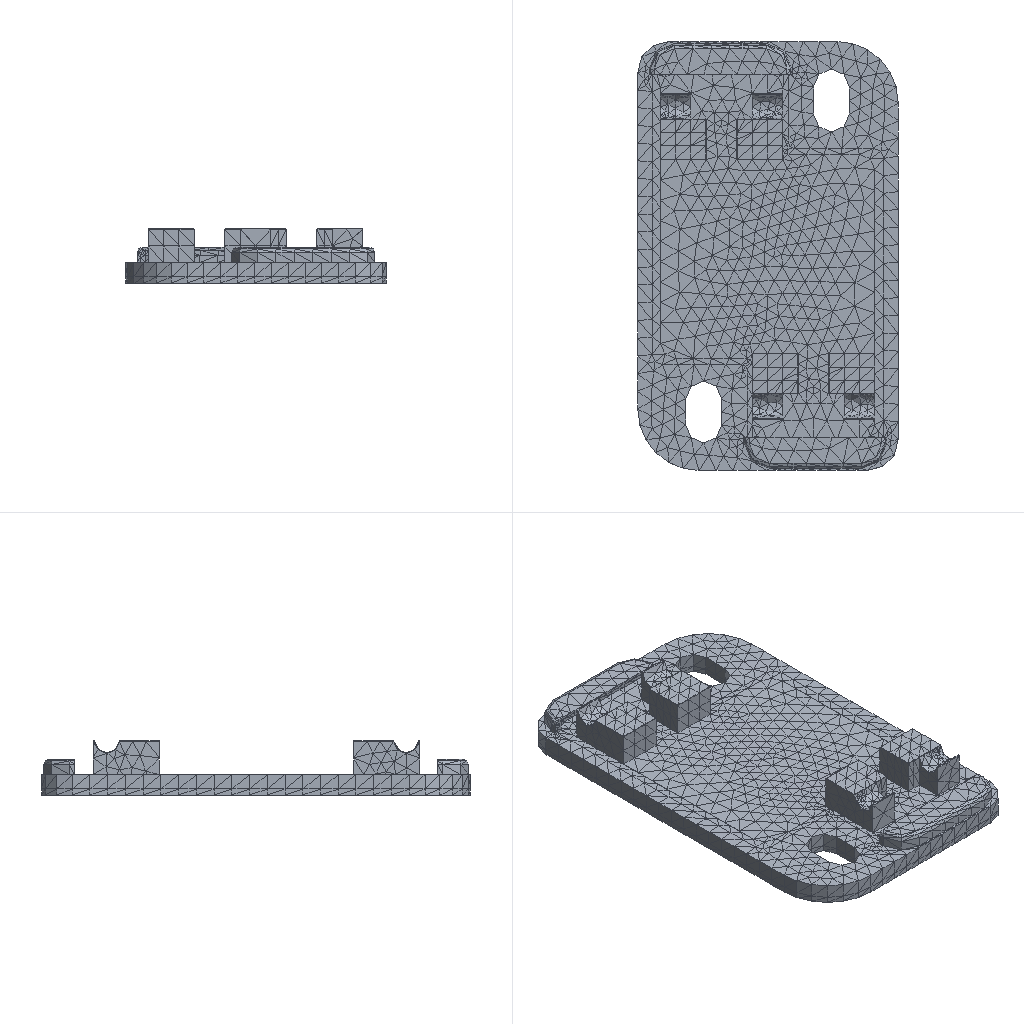Simulation study | abaqus
Set-up summary:
category,name,step,type,value,unit,region
solver,abaqus,,Abaqus/CAE 2024
units,mm-N-s-tonne (MPa),,inferred,E=2000 density=1e-09
analysis,Step-1,,frequency (modal),n_modes=100
mesh,nodes,,,20607
mesh,elements,,,10238
element_type,C3D10,,,9362
element_type,C3D8H,,,876
material,nilong,,E,2000
material,nilong,,nu,0.35
material,nilong,,density,1e-09
material,steel,,E,210000
material,steel,,nu,0.3
material,steel,,density,7.85e-09
material,xiangjiao,,density,1e-09
material,xiangjiao,,behaviors,hyperelastic
section,steel,,solid section,,,_PickedSet6
section,steel,,solid section,,,_PickedSet5
section,nilong,,solid section,,,_PickedSet5
section,xiangjiao,,solid section,,,_PickedSet3
bc,BC-1,initial,encastre,[dofs=ENCASTRE],,_PickedSet389
contact,CP-3-P1-3-1-P1-1-1,initial,tie,,,CP-5-P1-1-1 / CP-9-P1-3-1
contact,CP-4-P1-4-1-P1-1-1,initial,tie,,,CP-6-P1-1-1 / CP-4-P1-4-1
contact,CP-5-P1-3-1-P1-2-1,initial,tie,,,CP-7-P1-2-1 / CP-10-P1-3-1
contact,CP-6-P1-2-1-P1-3-1,initial,tie,,,CP-11-P1-3-1 / CP-8-P1-2-1
contact,CP-7-P1-3-1-P1-4-1,initial,tie,,,CP-7-P1-4-1 / CP-12-P1-3-1
Abaqus input file, long lists of numbers shortened:
*Heading
** Job name: deck Model name: 0429-Copy
** Generated by: Abaqus/CAE 2024
*Preprint, echo=NO, model=NO, history=NO, contact=NO
**
** PARTS
**
*Part, name=P1-1
*Node
      1,  -95.253,   153.152,   377.707
      2,  -95.253,   153.152,   377.707
** (9518 more lines like these left out)
*Element, type=C3D10
   1, 1289, 1290, 1291, 1292, 1562, 1561, 1560, 1564, 1563, 1565
   2, 1289,  471, 1290, 1293, 1567, 1566, 1562, 1569, 1568, 1570
** (5115 more lines like these left out)
*Nset, nset=_PickedSet6, internal, generate
    1,  9520,     1
*Elset, elset=_PickedSet6, internal, generate
    1,  5117,     1
** Section: Section-1
*Solid Section, elset=_PickedSet6, material=steel
,
*End Part
**
*Part, name=P1-2
*Node
      1,   6.642,  -185.857,         355.
      2,   6.642,  -183.857,         357.
** (4353 more lines like these left out)
*Element, type=C3D10
   1,  742,  660,   82,  656,  802,  801,  800,  804,  803,  805
   2,  742,  743,  660,  672,  807,  806,  802,  809,  808,  810
** (2008 more lines like these left out)
*Nset, nset=_PickedSet5, internal, generate
    1,  4355,     1
*Elset, elset=_PickedSet5, internal, generate
    1,  2010,     1
** Section: Section-1
*Solid Section, elset=_PickedSet5, material=steel
,
*End Part
**
*Part, name=P1-3
*Node
      1,   19.747,   198.648,         352.
      2,   19.747,   198.648,         357.
** (4880 more lines like these left out)
*Element, type=C3D10
   1,  293,  656,  715,   72,  894,  893,  892,  896,  895,  897
   2,  293,  860,   34,  656,  900,  899,  898,  894,  901,  902
** (2233 more lines like these left out)
*Nset, nset=_PickedSet5, internal, generate
    1,  4882,     1
*Elset, elset=_PickedSet5, internal, generate
    1,  2235,     1
** Section: Section-2
*Solid Section, elset=_PickedSet5, material=nilong
,
*End Part
**
*Part, name=P1-4
*Node
      1,  -10.923,  -83.852,         334.
      2,  -12.753,  -82.022,         334.
** (1848 more lines like these left out)
*Element, type=C3D8H
  1,  215,  234,  265,  226, 1140, 1159, 1190, 1151
  2,  591,    7,    6,  533, 1516,  932,  931, 1458
** (874 more lines like these left out)
*Nset, nset=_PickedSet3, internal, generate
    1,  1850,     1
*Elset, elset=_PickedSet3, internal, generate
   1,  876,    1
** Section: Section-3
*Solid Section, elset=_PickedSet3, material=xiangjiao
,
*End Part
**
**
** ASSEMBLY
**
*Assembly, name=Assembly
**
*Instance, name=P1-1-1, part=P1-1
*End Instance
**
*Instance, name=P1-2-1, part=P1-2
*End Instance
**
*Instance, name=P1-3-1, part=P1-3
*End Instance
**
*Instance, name=P1-4-1, part=P1-4
*End Instance
**
*Nset, nset=_PickedSet389, internal, instance=P1-2-1
   57,   58,   59,   60,   61,   62,   63,   64,  113,  114,  115,  116,  117,  118,  119,  120
  245,  246,  247,  248,  249,  250,  251,  252,  253,  254,  255,  256,  257,  258,  259,  260
** (26 more lines like these left out)
*Nset, nset=_PickedSet389, internal, instance=P1-3-1
   13,   14,   15,   16,   17,   18,   19,   20,   21,   22,   23,   24,   25,   26,   27,   28
   29,   30,   31,   32,   33,   34,   35,   36,   37,   38,   39,   40,   41,   42,   43,   44
** (57 more lines like these left out)
*Nset, nset=_PickedSet389, internal, instance=P1-4-1, generate
  926,  1850,     1
*Elset, elset=_PickedSet389, internal, instance=P1-2-1
   10,   18,   29,   33,   75,   84,   92,  120,  139,  150,  217,  229,  285,  323,  335,  383
  388,  424,  495,  508,  534,  544,  549,  556,  614,  618,  622,  625,  632,  636,  638,  643
** (8 more lines like these left out)
*Elset, elset=_PickedSet389, internal, instance=P1-3-1
    1,    2,   10,   42,   56,  110,  219,  232,  257,  263,  270,  277,  281,  288,  306,  341
  350,  355,  356,  388,  404,  405,  409,  419,  421,  432,  435,  451,  452,  463,  466,  468
** (22 more lines like these left out)
*Elset, elset=_PickedSet389, internal, instance=P1-4-1, generate
   1,  876,    1
*Elset, elset=_CP-1-P1-1-1_S1, internal, instance=P1-1-1
   90,  106,  129,  165,  230,  245,  306,  429,  598,  614,  660,  799,  815, 1067, 1087, 1092
 1125, 1176, 1221, 1393, 1458, 1462, 1652, 1679, 1712, 1818, 1850, 2003, 2019, 2196, 2311, 2440
** (3 more lines like these left out)
*Elset, elset=_CP-1-P1-1-1_S2, internal, instance=P1-1-1
   14,   22,   28,   92,  247,  248,  261,  301,  303,  323,  330,  375,  376,  429,  447,  448
  454,  578,  748,  751,  804,  888, 1223, 1356, 1357, 1358, 1511, 1559, 1644, 1684, 1733, 2822
** (5 more lines like these left out)
*Elset, elset=_CP-1-P1-1-1_S3, internal, instance=P1-1-1
   83,  164,  190,  204,  271,  279,  302,  327,  331,  339,  400,  451,  521,  522,  530,  560
  565,  599,  607,  617,  618,  637,  639,  697,  710,  715,  727,  769,  770,  771,  787,  791
** (32 more lines like these left out)
*Elset, elset=_CP-1-P1-1-1_S4, internal, instance=P1-1-1
   13,   80,  122,  139,  217,  256,  301,  348,  349,  353,  584,  586,  591,  707,  729,  812
  842,  880,  881,  900,  901,  922,  972,  989, 1030, 1130, 1243, 1246, 1330, 1341, 1373, 1406
** (7 more lines like these left out)
*Surface, type=ELEMENT, name=CP-1-P1-1-1
_CP-1-P1-1-1_S1, S1
_CP-1-P1-1-1_S2, S2
_CP-1-P1-1-1_S4, S4
_CP-1-P1-1-1_S3, S3
*Elset, elset=_CP-1-P1-3-1_S1, internal, instance=P1-3-1
   38,   45,  178,  234,  346,  748,  806,  810,  892, 1098, 1103, 1170, 1639, 1884, 1973, 1979
*Elset, elset=_CP-1-P1-3-1_S2, internal, instance=P1-3-1
  325,  347,  627,  747,  760,  761,  820,  897, 1082, 1097, 1100, 1129, 1165, 1177, 1961
*Elset, elset=_CP-1-P1-3-1_S4, internal, instance=P1-3-1
   21,   40,   47,   54,  733,  876,  889,  907,  920,  952,  953,  998, 1004, 1076, 1106, 1141
 1153, 1267, 1790, 1867
*Elset, elset=_CP-1-P1-3-1_S3, internal, instance=P1-3-1
    8,   25,   31,   92,  112,  134,  146,  162,  174,  231,  247,  714,  752,  812,  826,  839
  840,  860,  871,  891,  908,  913,  935,  961,  974, 1013, 1030, 1032, 1059, 1096, 1116, 1117
** (4 more lines like these left out)
*Surface, type=ELEMENT, name=CP-1-P1-3-1
_CP-1-P1-3-1_S1, S1
_CP-1-P1-3-1_S2, S2
_CP-1-P1-3-1_S4, S4
_CP-1-P1-3-1_S3, S3
*Elset, elset=_CP-2-P1-1-1_S1, internal, instance=P1-1-1
  141,  199,  470,  556,  755, 1260, 1527, 1570, 1645, 1692, 1716, 1731, 2123, 2167, 2219, 2303
 2328, 2329, 2515, 2567, 2613, 2734, 2865, 2880, 3055, 3129, 3234, 3243, 3256, 3259, 3345, 3400
** (3 more lines like these left out)
*Elset, elset=_CP-2-P1-1-1_S3, internal, instance=P1-1-1
  170,  173,  174,  273,  364,  481,  505,  587,  674,  678,  746,  756,  829,  905,  940, 1019
 1028, 1032, 1034, 1063, 1102, 1306, 1380, 1422, 1428, 1490, 1499, 1520, 1522, 1533, 1586, 1606
** (45 more lines like these left out)
*Elset, elset=_CP-2-P1-1-1_S4, internal, instance=P1-1-1
  194,  236,  454,  482,  921,  995, 1024, 1155, 1378, 1387, 1561, 1566, 1703, 1791, 1833, 1925
 1930, 1969, 2001, 2019, 2306, 2341, 2359, 2384, 2427, 2506, 2547, 2565, 2578, 2586, 2630, 2643
** (4 more lines like these left out)
*Elset, elset=_CP-2-P1-1-1_S2, internal, instance=P1-1-1
  474, 1563, 1607, 1982, 2200, 2468, 2584, 2596, 2714, 2777, 2789, 2842, 2848, 2853, 2859, 2871
 2916, 2944, 2973, 3004, 3007, 3022, 3045, 3056, 3067, 3153, 3156, 3158, 3188, 3351, 3357, 3378
** (3 more lines like these left out)
*Surface, type=ELEMENT, name=CP-2-P1-1-1
_CP-2-P1-1-1_S1, S1
_CP-2-P1-1-1_S3, S3
_CP-2-P1-1-1_S4, S4
_CP-2-P1-1-1_S2, S2
*Elset, elset=_CP-2-P1-3-1_S1, internal, instance=P1-3-1
   38,   45,  178,  234,  346,  748,  806,  810,  892, 1098, 1103, 1170, 1639, 1884, 1973, 1979
*Elset, elset=_CP-2-P1-3-1_S2, internal, instance=P1-3-1
  325,  347,  627,  747,  760,  761,  820,  897, 1082, 1097, 1100, 1129, 1165, 1177, 1961
*Elset, elset=_CP-2-P1-3-1_S4, internal, instance=P1-3-1
   21,   40,   47,   54,  733,  876,  889,  907,  920,  952,  953,  998, 1004, 1076, 1106, 1141
 1153, 1267, 1790, 1867
*Elset, elset=_CP-2-P1-3-1_S3, internal, instance=P1-3-1
    8,   25,   31,   92,  112,  134,  146,  162,  174,  231,  247,  714,  752,  812,  826,  839
  840,  860,  871,  891,  908,  913,  935,  961,  974, 1013, 1030, 1032, 1059, 1096, 1116, 1117
** (4 more lines like these left out)
*Surface, type=ELEMENT, name=CP-2-P1-3-1
_CP-2-P1-3-1_S1, S1
_CP-2-P1-3-1_S2, S2
_CP-2-P1-3-1_S4, S4
_CP-2-P1-3-1_S3, S3
*Elset, elset=_CP-2-P1-4-1_S1, internal, instance=P1-4-1, generate
   1,  876,    1
*Surface, type=ELEMENT, name=CP-2-P1-4-1
_CP-2-P1-4-1_S1, S1
*Elset, elset=_CP-3-P1-1-1_S1, internal, instance=P1-1-1
   90,  106,  129,  165,  230,  245,  306,  429,  598,  614,  660,  799,  815, 1067, 1087, 1092
 1125, 1176, 1221, 1393, 1458, 1462, 1652, 1679, 1712, 1818, 1850, 2003, 2019, 2196, 2311, 2440
** (3 more lines like these left out)
*Elset, elset=_CP-3-P1-1-1_S2, internal, instance=P1-1-1
   14,   22,   28,   92,  247,  248,  261,  301,  303,  323,  330,  375,  376,  429,  447,  448
  454,  578,  748,  751,  804,  888, 1223, 1356, 1357, 1358, 1511, 1559, 1644, 1684, 1733, 2822
** (5 more lines like these left out)
*Elset, elset=_CP-3-P1-1-1_S3, internal, instance=P1-1-1
   83,  164,  190,  204,  271,  279,  302,  327,  331,  339,  400,  451,  521,  522,  530,  560
  565,  599,  607,  617,  618,  637,  639,  697,  710,  715,  727,  769,  770,  771,  787,  791
** (32 more lines like these left out)
*Elset, elset=_CP-3-P1-1-1_S4, internal, instance=P1-1-1
   13,   80,  122,  139,  217,  256,  301,  348,  349,  353,  584,  586,  591,  707,  729,  812
  842,  880,  881,  900,  901,  922,  972,  989, 1030, 1130, 1243, 1246, 1330, 1341, 1373, 1406
** (7 more lines like these left out)
*Surface, type=ELEMENT, name=CP-3-P1-1-1
_CP-3-P1-1-1_S1, S1
_CP-3-P1-1-1_S2, S2
_CP-3-P1-1-1_S4, S4
_CP-3-P1-1-1_S3, S3
*Elset, elset=_CP-3-P1-2-1_S3, internal, instance=P1-2-1
   13,   45,   65,   79,   81,   91,  104,  118,  138,  146,  152,  154,  172,  204,  210,  227
  232,  235,  249,  268,  282,  321,  377,  446,  449,  484,  497,  511,  526,  550,  576,  578
** (11 more lines like these left out)
*Elset, elset=_CP-3-P1-2-1_S2, internal, instance=P1-2-1
    4,  277,  367,  370,  460,  461,  464,  726,  781,  843,  874,  922,  961, 1036, 1057, 1083
 1093, 1384, 1438, 1439, 1457, 1466, 1560, 1570, 1588, 1627, 1730, 1756, 1809, 1839, 1855, 1858
** (1 more lines like these left out)
*Elset, elset=_CP-3-P1-2-1_S4, internal, instance=P1-2-1
  279,  344,  485,  647,  649,  650,  749,  888,  890,  891,  894,  936,  977, 1013, 1018, 1022
 1042, 1058, 1131, 1135, 1169, 1180, 1187, 1231, 1235, 1258, 1290, 1295, 1333, 1334, 1345, 1354
** (3 more lines like these left out)
*Elset, elset=_CP-3-P1-2-1_S1, internal, instance=P1-2-1
  134,  212,  213,  267,  274,  342,  478,  872,  972, 1050, 1094, 1128, 1451, 1477, 1534, 1555
 1578, 1591, 1598, 1611, 1645, 1693, 1704, 1712, 1726, 1734, 1737, 1787, 1834, 1847, 1848, 1875
** (1 more lines like these left out)
*Surface, type=ELEMENT, name=CP-3-P1-2-1
_CP-3-P1-2-1_S3, S3
_CP-3-P1-2-1_S2, S2
_CP-3-P1-2-1_S4, S4
_CP-3-P1-2-1_S1, S1
*Elset, elset=_CP-3-P1-3-1_S3, internal, instance=P1-3-1
   35,   36,   72,   75,   78,  180,  181,  192,  218,  221,  225,  240,  251,  429,  521,  536
  603,  607,  618,  633,  670,  783,  784,  799,  819,  859,  864,  906,  921,  926,  933,  958
** (3 more lines like these left out)
*Elset, elset=_CP-3-P1-3-1_S4, internal, instance=P1-3-1
   61,  138,  153,  159,  195,  200,  202,  206,  233,  239,  260,  370,  493,  516,  520,  525
  526,  533,  538,  545,  546,  550,  558,  569,  573,  574,  580,  586,  591,  608,  611,  615
** (4 more lines like these left out)
*Elset, elset=_CP-3-P1-3-1_S2, internal, instance=P1-3-1
   14,  196,  203,  210,  212,  213,  245,  246,  249,  252,  512,  515,  529,  541,  555,  566
  567,  570,  571,  576,  583,  585,  588,  625,  645,  652,  676,  677,  690,  694,  701,  713
** (5 more lines like these left out)
*Elset, elset=_CP-3-P1-3-1_S1, internal, instance=P1-3-1
   13,   98,  122,  154,  194,  265,  327,  351,  456,  517,  524,  535,  554,  557,  564,  584
  605,  619,  634,  635,  660,  679,  680,  686,  697,  708,  721,  728,  745,  750,  772,  789
** (4 more lines like these left out)
*Surface, type=ELEMENT, name=CP-3-P1-3-1
_CP-3-P1-3-1_S3, S3
_CP-3-P1-3-1_S4, S4
_CP-3-P1-3-1_S2, S2
_CP-3-P1-3-1_S1, S1
*Elset, elset=_CP-3-P1-4-1_S1, internal, instance=P1-4-1, generate
   1,  876,    1
*Surface, type=ELEMENT, name=CP-3-P1-4-1
_CP-3-P1-4-1_S1, S1
*Elset, elset=_CP-4-P1-1-1_S1, internal, instance=P1-1-1
  141,  199,  470,  556,  755, 1260, 1527, 1570, 1645, 1692, 1716, 1731, 2123, 2167, 2219, 2303
 2328, 2329, 2515, 2567, 2613, 2734, 2865, 2880, 3055, 3129, 3234, 3243, 3256, 3259, 3345, 3400
** (3 more lines like these left out)
*Elset, elset=_CP-4-P1-1-1_S3, internal, instance=P1-1-1
  170,  173,  174,  273,  364,  481,  505,  587,  674,  678,  746,  756,  829,  905,  940, 1019
 1028, 1032, 1034, 1063, 1102, 1306, 1380, 1422, 1428, 1490, 1499, 1520, 1522, 1533, 1586, 1606
** (45 more lines like these left out)
*Elset, elset=_CP-4-P1-1-1_S4, internal, instance=P1-1-1
  194,  236,  454,  482,  921,  995, 1024, 1155, 1378, 1387, 1561, 1566, 1703, 1791, 1833, 1925
 1930, 1969, 2001, 2019, 2306, 2341, 2359, 2384, 2427, 2506, 2547, 2565, 2578, 2586, 2630, 2643
** (4 more lines like these left out)
*Elset, elset=_CP-4-P1-1-1_S2, internal, instance=P1-1-1
  474, 1563, 1607, 1982, 2200, 2468, 2584, 2596, 2714, 2777, 2789, 2842, 2848, 2853, 2859, 2871
 2916, 2944, 2973, 3004, 3007, 3022, 3045, 3056, 3067, 3153, 3156, 3158, 3188, 3351, 3357, 3378
** (3 more lines like these left out)
*Surface, type=ELEMENT, name=CP-4-P1-1-1
_CP-4-P1-1-1_S1, S1
_CP-4-P1-1-1_S3, S3
_CP-4-P1-1-1_S4, S4
_CP-4-P1-1-1_S2, S2
*Elset, elset=_CP-4-P1-2-1_S4, internal, instance=P1-2-1
    4,  216,  280,  350,  367,  408,  419,  478,  491,  553,  582,  584,  652,  659,  683,  765
  768,  866,  874,  931,  963, 1095, 1106, 1126, 1129, 1166, 1241, 1243, 1263, 1279, 1292, 1313
** (1 more lines like these left out)
*Elset, elset=_CP-4-P1-2-1_S3, internal, instance=P1-2-1
    8,   29,  109,  174,  238,  281,  287,  296,  316,  356,  426,  429,  462,  473,  488,  523
  529,  531,  542,  574,  620,  661,  668,  669,  705,  711,  742,  744,  745,  747,  749,  759
** (12 more lines like these left out)
*Elset, elset=_CP-4-P1-2-1_S1, internal, instance=P1-2-1
  224,  374,  611,  643,  660,  678,  693,  725,  946,  991, 1042, 1133, 1265, 1306, 1339
*Elset, elset=_CP-4-P1-2-1_S2, internal, instance=P1-2-1
  303,  539,  772,  867,  897,  948,  967, 1026, 1030, 1089, 1137, 1172, 1175, 1176, 1200, 1215
 1221, 1228, 1252, 1260, 1264, 1288, 1301, 1332, 1354, 1369, 1435, 1461, 1472, 1732, 1764, 1821
** (1 more lines like these left out)
*Surface, type=ELEMENT, name=CP-4-P1-2-1
_CP-4-P1-2-1_S4, S4
_CP-4-P1-2-1_S3, S3
_CP-4-P1-2-1_S2, S2
_CP-4-P1-2-1_S1, S1
*Elset, elset=_CP-4-P1-3-1_S1, internal, instance=P1-3-1
  255,  261,  292,  302,  304,  307,  320,  330,  343,  363,  368,  383,  395,  400,  433,  454
  464,  478,  481,  486,  781,  787,  843,  895,  955,  967,  970,  999, 1012, 1111, 1113, 1130
** (5 more lines like these left out)
*Elset, elset=_CP-4-P1-3-1_S4, internal, instance=P1-3-1
  258,  279,  291,  298,  305,  324,  331,  338,  372,  394,  401,  408,  411,  422,  423,  444
  445,  487,  490,  499,  575,  681,  778,  800,  807,  827,  851,  862,  877,  930,  938,  939
** (3 more lines like these left out)
*Elset, elset=_CP-4-P1-3-1_S2, internal, instance=P1-3-1
  259,  268,  271,  273,  282,  286,  287,  293,  294,  299,  313,  321,  329,  333,  334,  349
  357,  366,  371,  378,  381,  382,  396,  406,  415,  417,  418,  441,  442,  443,  455,  458
** (5 more lines like these left out)
*Elset, elset=_CP-4-P1-3-1_S3, internal, instance=P1-3-1
  312,  390,  398,  440,  447,  491,  500,  514,  925, 1164, 1183, 1286, 1287, 1352, 1362, 1389
 1437, 1559, 1780, 1783, 1802, 1847, 2170
*Surface, type=ELEMENT, name=CP-4-P1-3-1
_CP-4-P1-3-1_S1, S1
_CP-4-P1-3-1_S4, S4
_CP-4-P1-3-1_S2, S2
_CP-4-P1-3-1_S3, S3
*Elset, elset=_CP-4-P1-4-1_S1, internal, instance=P1-4-1, generate
   1,  876,    1
*Surface, type=ELEMENT, name=CP-4-P1-4-1
_CP-4-P1-4-1_S1, S1
*Elset, elset=_CP-5-P1-1-1_S1, internal, instance=P1-1-1
   90,  106,  129,  165,  230,  245,  306,  429,  598,  614,  660,  799,  815, 1067, 1087, 1092
 1125, 1176, 1221, 1393, 1458, 1462, 1652, 1679, 1712, 1818, 1850, 2003, 2019, 2196, 2311, 2440
** (3 more lines like these left out)
*Elset, elset=_CP-5-P1-1-1_S2, internal, instance=P1-1-1
   14,   22,   28,   92,  247,  248,  261,  301,  303,  323,  330,  375,  376,  429,  447,  448
  454,  578,  748,  751,  804,  888, 1223, 1356, 1357, 1358, 1511, 1559, 1644, 1684, 1733, 2822
** (5 more lines like these left out)
*Elset, elset=_CP-5-P1-1-1_S3, internal, instance=P1-1-1
   83,  164,  190,  204,  271,  279,  302,  327,  331,  339,  400,  451,  521,  522,  530,  560
  565,  599,  607,  617,  618,  637,  639,  697,  710,  715,  727,  769,  770,  771,  787,  791
** (32 more lines like these left out)
*Elset, elset=_CP-5-P1-1-1_S4, internal, instance=P1-1-1
   13,   80,  122,  139,  217,  256,  301,  348,  349,  353,  584,  586,  591,  707,  729,  812
  842,  880,  881,  900,  901,  922,  972,  989, 1030, 1130, 1243, 1246, 1330, 1341, 1373, 1406
** (7 more lines like these left out)
*Surface, type=ELEMENT, name=CP-5-P1-1-1
_CP-5-P1-1-1_S1, S1
_CP-5-P1-1-1_S2, S2
_CP-5-P1-1-1_S4, S4
_CP-5-P1-1-1_S3, S3
*Elset, elset=_CP-5-P1-2-1_S3, internal, instance=P1-2-1
   13,   45,   65,   79,   81,   91,  104,  118,  138,  146,  152,  154,  172,  204,  210,  227
  232,  235,  249,  268,  282,  321,  377,  446,  449,  484,  497,  511,  526,  550,  576,  578
** (11 more lines like these left out)
*Elset, elset=_CP-5-P1-2-1_S2, internal, instance=P1-2-1
    4,  277,  367,  370,  460,  461,  464,  726,  781,  843,  874,  922,  961, 1036, 1057, 1083
 1093, 1384, 1438, 1439, 1457, 1466, 1560, 1570, 1588, 1627, 1730, 1756, 1809, 1839, 1855, 1858
** (1 more lines like these left out)
*Elset, elset=_CP-5-P1-2-1_S4, internal, instance=P1-2-1
  279,  344,  485,  647,  649,  650,  749,  888,  890,  891,  894,  936,  977, 1013, 1018, 1022
 1042, 1058, 1131, 1135, 1169, 1180, 1187, 1231, 1235, 1258, 1290, 1295, 1333, 1334, 1345, 1354
** (3 more lines like these left out)
*Elset, elset=_CP-5-P1-2-1_S1, internal, instance=P1-2-1
  134,  212,  213,  267,  274,  342,  478,  872,  972, 1050, 1094, 1128, 1451, 1477, 1534, 1555
 1578, 1591, 1598, 1611, 1645, 1693, 1704, 1712, 1726, 1734, 1737, 1787, 1834, 1847, 1848, 1875
** (1 more lines like these left out)
*Surface, type=ELEMENT, name=CP-5-P1-2-1
_CP-5-P1-2-1_S3, S3
_CP-5-P1-2-1_S2, S2
_CP-5-P1-2-1_S4, S4
_CP-5-P1-2-1_S1, S1
*Elset, elset=_CP-5-P1-3-1_S1, internal, instance=P1-3-1
   38,   45,  178,  234,  346,  748,  806,  810,  892, 1098, 1103, 1170, 1639, 1884, 1973, 1979
*Elset, elset=_CP-5-P1-3-1_S2, internal, instance=P1-3-1
  325,  347,  627,  747,  760,  761,  820,  897, 1082, 1097, 1100, 1129, 1165, 1177, 1961
*Elset, elset=_CP-5-P1-3-1_S4, internal, instance=P1-3-1
   21,   40,   47,   54,  733,  876,  889,  907,  920,  952,  953,  998, 1004, 1076, 1106, 1141
 1153, 1267, 1790, 1867
*Elset, elset=_CP-5-P1-3-1_S3, internal, instance=P1-3-1
    8,   25,   31,   92,  112,  134,  146,  162,  174,  231,  247,  714,  752,  812,  826,  839
  840,  860,  871,  891,  908,  913,  935,  961,  974, 1013, 1030, 1032, 1059, 1096, 1116, 1117
** (4 more lines like these left out)
*Surface, type=ELEMENT, name=CP-5-P1-3-1
_CP-5-P1-3-1_S1, S1
_CP-5-P1-3-1_S2, S2
_CP-5-P1-3-1_S4, S4
_CP-5-P1-3-1_S3, S3
*Elset, elset=_CP-5-P1-4-1_S3, internal, instance=P1-4-1
   3,   7,  18, 169, 225, 286, 317, 382, 417, 446, 449, 492, 524, 531, 541, 544
 545, 550, 555, 563, 576, 616, 625, 626
*Elset, elset=_CP-5-P1-4-1_S4, internal, instance=P1-4-1
   2,  11,  14,  33,  74,  79,  82,  84, 140, 162, 273, 313, 538, 567, 568, 570
 573, 574, 577, 588, 590, 592, 634, 635
*Elset, elset=_CP-5-P1-4-1_S5, internal, instance=P1-4-1
   5,   9,  26,  27,  32,  58,  81, 112, 142, 260, 282, 325, 368, 579, 596, 601
 602, 609, 623, 844
*Elset, elset=_CP-5-P1-4-1_S6, internal, instance=P1-4-1
   5,  13,  17,  25,  50,  54,  57,  58, 210, 248, 277, 456, 465, 496, 519, 522
 528, 551, 558, 559, 560, 561, 565, 575, 583, 622, 632, 844
*Surface, type=ELEMENT, name=CP-5-P1-4-1
_CP-5-P1-4-1_S3, S3
_CP-5-P1-4-1_S4, S4
_CP-5-P1-4-1_S6, S6
_CP-5-P1-4-1_S5, S5
*Elset, elset=_CP-6-P1-1-1_S1, internal, instance=P1-1-1
  141,  199,  470,  556,  755, 1260, 1527, 1570, 1645, 1692, 1716, 1731, 2123, 2167, 2219, 2303
 2328, 2329, 2515, 2567, 2613, 2734, 2865, 2880, 3055, 3129, 3234, 3243, 3256, 3259, 3345, 3400
** (3 more lines like these left out)
*Elset, elset=_CP-6-P1-1-1_S3, internal, instance=P1-1-1
  170,  173,  174,  273,  364,  481,  505,  587,  674,  678,  746,  756,  829,  905,  940, 1019
 1028, 1032, 1034, 1063, 1102, 1306, 1380, 1422, 1428, 1490, 1499, 1520, 1522, 1533, 1586, 1606
** (45 more lines like these left out)
*Elset, elset=_CP-6-P1-1-1_S4, internal, instance=P1-1-1
  194,  236,  454,  482,  921,  995, 1024, 1155, 1378, 1387, 1561, 1566, 1703, 1791, 1833, 1925
 1930, 1969, 2001, 2019, 2306, 2341, 2359, 2384, 2427, 2506, 2547, 2565, 2578, 2586, 2630, 2643
** (4 more lines like these left out)
*Elset, elset=_CP-6-P1-1-1_S2, internal, instance=P1-1-1
  474, 1563, 1607, 1982, 2200, 2468, 2584, 2596, 2714, 2777, 2789, 2842, 2848, 2853, 2859, 2871
 2916, 2944, 2973, 3004, 3007, 3022, 3045, 3056, 3067, 3153, 3156, 3158, 3188, 3351, 3357, 3378
** (3 more lines like these left out)
*Surface, type=ELEMENT, name=CP-6-P1-1-1
_CP-6-P1-1-1_S1, S1
_CP-6-P1-1-1_S3, S3
_CP-6-P1-1-1_S4, S4
_CP-6-P1-1-1_S2, S2
*Elset, elset=_CP-6-P1-2-1_S4, internal, instance=P1-2-1
    4,  216,  280,  350,  367,  408,  419,  478,  491,  553,  582,  584,  652,  659,  683,  765
  768,  866,  874,  931,  963, 1095, 1106, 1126, 1129, 1166, 1241, 1243, 1263, 1279, 1292, 1313
** (1 more lines like these left out)
*Elset, elset=_CP-6-P1-2-1_S3, internal, instance=P1-2-1
    8,   29,  109,  174,  238,  281,  287,  296,  316,  356,  426,  429,  462,  473,  488,  523
  529,  531,  542,  574,  620,  661,  668,  669,  705,  711,  742,  744,  745,  747,  749,  759
** (12 more lines like these left out)
*Elset, elset=_CP-6-P1-2-1_S1, internal, instance=P1-2-1
  224,  374,  611,  643,  660,  678,  693,  725,  946,  991, 1042, 1133, 1265, 1306, 1339
*Elset, elset=_CP-6-P1-2-1_S2, internal, instance=P1-2-1
  303,  539,  772,  867,  897,  948,  967, 1026, 1030, 1089, 1137, 1172, 1175, 1176, 1200, 1215
 1221, 1228, 1252, 1260, 1264, 1288, 1301, 1332, 1354, 1369, 1435, 1461, 1472, 1732, 1764, 1821
** (1 more lines like these left out)
*Surface, type=ELEMENT, name=CP-6-P1-2-1
_CP-6-P1-2-1_S4, S4
_CP-6-P1-2-1_S3, S3
_CP-6-P1-2-1_S2, S2
_CP-6-P1-2-1_S1, S1
*Elset, elset=_CP-6-P1-3-1_S3, internal, instance=P1-3-1
   35,   36,   72,   75,   78,  180,  181,  192,  218,  221,  225,  240,  251,  429,  521,  536
  603,  607,  618,  633,  670,  783,  784,  799,  819,  859,  864,  906,  921,  926,  933,  958
** (3 more lines like these left out)
*Elset, elset=_CP-6-P1-3-1_S4, internal, instance=P1-3-1
   61,  138,  153,  159,  195,  200,  202,  206,  233,  239,  260,  370,  493,  516,  520,  525
  526,  533,  538,  545,  546,  550,  558,  569,  573,  574,  580,  586,  591,  608,  611,  615
** (4 more lines like these left out)
*Elset, elset=_CP-6-P1-3-1_S2, internal, instance=P1-3-1
   14,  196,  203,  210,  212,  213,  245,  246,  249,  252,  512,  515,  529,  541,  555,  566
  567,  570,  571,  576,  583,  585,  588,  625,  645,  652,  676,  677,  690,  694,  701,  713
** (5 more lines like these left out)
*Elset, elset=_CP-6-P1-3-1_S1, internal, instance=P1-3-1
   13,   98,  122,  154,  194,  265,  327,  351,  456,  517,  524,  535,  554,  557,  564,  584
  605,  619,  634,  635,  660,  679,  680,  686,  697,  708,  721,  728,  745,  750,  772,  789
** (4 more lines like these left out)
*Surface, type=ELEMENT, name=CP-6-P1-3-1
_CP-6-P1-3-1_S3, S3
_CP-6-P1-3-1_S4, S4
_CP-6-P1-3-1_S2, S2
_CP-6-P1-3-1_S1, S1
*Elset, elset=_CP-6-P1-4-1_S3, internal, instance=P1-4-1
   3,   7,  18, 169, 225, 286, 317, 382, 417, 446, 449, 492, 524, 531, 541, 544
 545, 550, 555, 563, 576, 616, 625, 626
*Elset, elset=_CP-6-P1-4-1_S4, internal, instance=P1-4-1
   2,  11,  14,  33,  74,  79,  82,  84, 140, 162, 273, 313, 538, 567, 568, 570
 573, 574, 577, 588, 590, 592, 634, 635
*Elset, elset=_CP-6-P1-4-1_S5, internal, instance=P1-4-1
   5,   9,  26,  27,  32,  58,  81, 112, 142, 260, 282, 325, 368, 579, 596, 601
 602, 609, 623, 844
*Elset, elset=_CP-6-P1-4-1_S6, internal, instance=P1-4-1
   5,  13,  17,  25,  50,  54,  57,  58, 210, 248, 277, 456, 465, 496, 519, 522
 528, 551, 558, 559, 560, 561, 565, 575, 583, 622, 632, 844
*Surface, type=ELEMENT, name=CP-6-P1-4-1
_CP-6-P1-4-1_S3, S3
_CP-6-P1-4-1_S4, S4
_CP-6-P1-4-1_S6, S6
_CP-6-P1-4-1_S5, S5
*Elset, elset=_CP-7-P1-2-1_S3, internal, instance=P1-2-1
   13,   45,   65,   79,   81,   91,  104,  118,  138,  146,  152,  154,  172,  204,  210,  227
  232,  235,  249,  268,  282,  321,  377,  446,  449,  484,  497,  511,  526,  550,  576,  578
** (11 more lines like these left out)
*Elset, elset=_CP-7-P1-2-1_S2, internal, instance=P1-2-1
    4,  277,  367,  370,  460,  461,  464,  726,  781,  843,  874,  922,  961, 1036, 1057, 1083
 1093, 1384, 1438, 1439, 1457, 1466, 1560, 1570, 1588, 1627, 1730, 1756, 1809, 1839, 1855, 1858
** (1 more lines like these left out)
*Elset, elset=_CP-7-P1-2-1_S4, internal, instance=P1-2-1
  279,  344,  485,  647,  649,  650,  749,  888,  890,  891,  894,  936,  977, 1013, 1018, 1022
 1042, 1058, 1131, 1135, 1169, 1180, 1187, 1231, 1235, 1258, 1290, 1295, 1333, 1334, 1345, 1354
** (3 more lines like these left out)
*Elset, elset=_CP-7-P1-2-1_S1, internal, instance=P1-2-1
  134,  212,  213,  267,  274,  342,  478,  872,  972, 1050, 1094, 1128, 1451, 1477, 1534, 1555
 1578, 1591, 1598, 1611, 1645, 1693, 1704, 1712, 1726, 1734, 1737, 1787, 1834, 1847, 1848, 1875
** (1 more lines like these left out)
*Surface, type=ELEMENT, name=CP-7-P1-2-1
_CP-7-P1-2-1_S3, S3
_CP-7-P1-2-1_S2, S2
_CP-7-P1-2-1_S4, S4
_CP-7-P1-2-1_S1, S1
*Elset, elset=_CP-7-P1-3-1_S1, internal, instance=P1-3-1
  255,  261,  292,  302,  304,  307,  320,  330,  343,  363,  368,  383,  395,  400,  433,  454
  464,  478,  481,  486,  781,  787,  843,  895,  955,  967,  970,  999, 1012, 1111, 1113, 1130
** (5 more lines like these left out)
*Elset, elset=_CP-7-P1-3-1_S4, internal, instance=P1-3-1
  258,  279,  291,  298,  305,  324,  331,  338,  372,  394,  401,  408,  411,  422,  423,  444
  445,  487,  490,  499,  575,  681,  778,  800,  807,  827,  851,  862,  877,  930,  938,  939
** (3 more lines like these left out)
*Elset, elset=_CP-7-P1-3-1_S2, internal, instance=P1-3-1
  259,  268,  271,  273,  282,  286,  287,  293,  294,  299,  313,  321,  329,  333,  334,  349
  357,  366,  371,  378,  381,  382,  396,  406,  415,  417,  418,  441,  442,  443,  455,  458
** (5 more lines like these left out)
*Elset, elset=_CP-7-P1-3-1_S3, internal, instance=P1-3-1
  312,  390,  398,  440,  447,  491,  500,  514,  925, 1164, 1183, 1286, 1287, 1352, 1362, 1389
 1437, 1559, 1780, 1783, 1802, 1847, 2170
*Surface, type=ELEMENT, name=CP-7-P1-3-1
_CP-7-P1-3-1_S1, S1
_CP-7-P1-3-1_S4, S4
_CP-7-P1-3-1_S2, S2
_CP-7-P1-3-1_S3, S3
*Elset, elset=_CP-7-P1-4-1_S3, internal, instance=P1-4-1
   3,   7,  18, 169, 225, 286, 317, 382, 417, 446, 449, 492, 524, 531, 541, 544
 545, 550, 555, 563, 576, 616, 625, 626
*Elset, elset=_CP-7-P1-4-1_S4, internal, instance=P1-4-1
   2,  11,  14,  33,  74,  79,  82,  84, 140, 162, 273, 313, 538, 567, 568, 570
 573, 574, 577, 588, 590, 592, 634, 635
*Elset, elset=_CP-7-P1-4-1_S5, internal, instance=P1-4-1
   5,   9,  26,  27,  32,  58,  81, 112, 142, 260, 282, 325, 368, 579, 596, 601
 602, 609, 623, 844
*Elset, elset=_CP-7-P1-4-1_S6, internal, instance=P1-4-1
   5,  13,  17,  25,  50,  54,  57,  58, 210, 248, 277, 456, 465, 496, 519, 522
 528, 551, 558, 559, 560, 561, 565, 575, 583, 622, 632, 844
*Surface, type=ELEMENT, name=CP-7-P1-4-1
_CP-7-P1-4-1_S3, S3
_CP-7-P1-4-1_S4, S4
_CP-7-P1-4-1_S6, S6
_CP-7-P1-4-1_S5, S5
*Elset, elset=_CP-8-P1-2-1_S4, internal, instance=P1-2-1
    4,  216,  280,  350,  367,  408,  419,  478,  491,  553,  582,  584,  652,  659,  683,  765
  768,  866,  874,  931,  963, 1095, 1106, 1126, 1129, 1166, 1241, 1243, 1263, 1279, 1292, 1313
** (1 more lines like these left out)
*Elset, elset=_CP-8-P1-2-1_S3, internal, instance=P1-2-1
    8,   29,  109,  174,  238,  281,  287,  296,  316,  356,  426,  429,  462,  473,  488,  523
  529,  531,  542,  574,  620,  661,  668,  669,  705,  711,  742,  744,  745,  747,  749,  759
** (12 more lines like these left out)
*Elset, elset=_CP-8-P1-2-1_S1, internal, instance=P1-2-1
  224,  374,  611,  643,  660,  678,  693,  725,  946,  991, 1042, 1133, 1265, 1306, 1339
*Elset, elset=_CP-8-P1-2-1_S2, internal, instance=P1-2-1
  303,  539,  772,  867,  897,  948,  967, 1026, 1030, 1089, 1137, 1172, 1175, 1176, 1200, 1215
 1221, 1228, 1252, 1260, 1264, 1288, 1301, 1332, 1354, 1369, 1435, 1461, 1472, 1732, 1764, 1821
** (1 more lines like these left out)
*Surface, type=ELEMENT, name=CP-8-P1-2-1
_CP-8-P1-2-1_S4, S4
_CP-8-P1-2-1_S3, S3
_CP-8-P1-2-1_S2, S2
_CP-8-P1-2-1_S1, S1
*Elset, elset=_CP-8-P1-3-1_S1, internal, instance=P1-3-1
   38,   45,  178,  234,  346,  748,  806,  810,  892, 1098, 1103, 1170, 1639, 1884, 1973, 1979
*Elset, elset=_CP-8-P1-3-1_S2, internal, instance=P1-3-1
  325,  347,  627,  747,  760,  761,  820,  897, 1082, 1097, 1100, 1129, 1165, 1177, 1961
*Elset, elset=_CP-8-P1-3-1_S4, internal, instance=P1-3-1
   21,   40,   47,   54,  733,  876,  889,  907,  920,  952,  953,  998, 1004, 1076, 1106, 1141
 1153, 1267, 1790, 1867
*Elset, elset=_CP-8-P1-3-1_S3, internal, instance=P1-3-1
    8,   25,   31,   92,  112,  134,  146,  162,  174,  231,  247,  714,  752,  812,  826,  839
  840,  860,  871,  891,  908,  913,  935,  961,  974, 1013, 1030, 1032, 1059, 1096, 1116, 1117
** (4 more lines like these left out)
*Surface, type=ELEMENT, name=CP-8-P1-3-1
_CP-8-P1-3-1_S1, S1
_CP-8-P1-3-1_S2, S2
_CP-8-P1-3-1_S4, S4
_CP-8-P1-3-1_S3, S3
*Elset, elset=_CP-9-P1-3-1_S1, internal, instance=P1-3-1
   38,   45,  178,  234,  346,  748,  806,  810,  892, 1098, 1103, 1170, 1639, 1884, 1973, 1979
*Elset, elset=_CP-9-P1-3-1_S2, internal, instance=P1-3-1
  325,  347,  627,  747,  760,  761,  820,  897, 1082, 1097, 1100, 1129, 1165, 1177, 1961
*Elset, elset=_CP-9-P1-3-1_S4, internal, instance=P1-3-1
   21,   40,   47,   54,  733,  876,  889,  907,  920,  952,  953,  998, 1004, 1076, 1106, 1141
 1153, 1267, 1790, 1867
*Elset, elset=_CP-9-P1-3-1_S3, internal, instance=P1-3-1
    8,   25,   31,   92,  112,  134,  146,  162,  174,  231,  247,  714,  752,  812,  826,  839
  840,  860,  871,  891,  908,  913,  935,  961,  974, 1013, 1030, 1032, 1059, 1096, 1116, 1117
** (4 more lines like these left out)
*Surface, type=ELEMENT, name=CP-9-P1-3-1
_CP-9-P1-3-1_S1, S1
_CP-9-P1-3-1_S2, S2
_CP-9-P1-3-1_S4, S4
_CP-9-P1-3-1_S3, S3
*Elset, elset=_CP-10-P1-3-1_S3, internal, instance=P1-3-1
   35,   36,   72,   75,   78,  180,  181,  192,  218,  221,  225,  240,  251,  429,  521,  536
  603,  607,  618,  633,  670,  783,  784,  799,  819,  859,  864,  906,  921,  926,  933,  958
** (3 more lines like these left out)
*Elset, elset=_CP-10-P1-3-1_S4, internal, instance=P1-3-1
   61,  138,  153,  159,  195,  200,  202,  206,  233,  239,  260,  370,  493,  516,  520,  525
  526,  533,  538,  545,  546,  550,  558,  569,  573,  574,  580,  586,  591,  608,  611,  615
** (4 more lines like these left out)
*Elset, elset=_CP-10-P1-3-1_S2, internal, instance=P1-3-1
   14,  196,  203,  210,  212,  213,  245,  246,  249,  252,  512,  515,  529,  541,  555,  566
  567,  570,  571,  576,  583,  585,  588,  625,  645,  652,  676,  677,  690,  694,  701,  713
** (5 more lines like these left out)
*Elset, elset=_CP-10-P1-3-1_S1, internal, instance=P1-3-1
   13,   98,  122,  154,  194,  265,  327,  351,  456,  517,  524,  535,  554,  557,  564,  584
  605,  619,  634,  635,  660,  679,  680,  686,  697,  708,  721,  728,  745,  750,  772,  789
** (4 more lines like these left out)
*Surface, type=ELEMENT, name=CP-10-P1-3-1
_CP-10-P1-3-1_S3, S3
_CP-10-P1-3-1_S4, S4
_CP-10-P1-3-1_S2, S2
_CP-10-P1-3-1_S1, S1
*Elset, elset=_CP-11-P1-3-1_S1, internal, instance=P1-3-1
  255,  261,  292,  302,  304,  307,  320,  330,  343,  363,  368,  383,  395,  400,  433,  454
  464,  478,  481,  486,  781,  787,  843,  895,  955,  967,  970,  999, 1012, 1111, 1113, 1130
** (5 more lines like these left out)
*Elset, elset=_CP-11-P1-3-1_S4, internal, instance=P1-3-1
  258,  279,  291,  298,  305,  324,  331,  338,  372,  394,  401,  408,  411,  422,  423,  444
  445,  487,  490,  499,  575,  681,  778,  800,  807,  827,  851,  862,  877,  930,  938,  939
** (3 more lines like these left out)
*Elset, elset=_CP-11-P1-3-1_S2, internal, instance=P1-3-1
  259,  268,  271,  273,  282,  286,  287,  293,  294,  299,  313,  321,  329,  333,  334,  349
  357,  366,  371,  378,  381,  382,  396,  406,  415,  417,  418,  441,  442,  443,  455,  458
** (5 more lines like these left out)
*Elset, elset=_CP-11-P1-3-1_S3, internal, instance=P1-3-1
  312,  390,  398,  440,  447,  491,  500,  514,  925, 1164, 1183, 1286, 1287, 1352, 1362, 1389
 1437, 1559, 1780, 1783, 1802, 1847, 2170
*Surface, type=ELEMENT, name=CP-11-P1-3-1
_CP-11-P1-3-1_S1, S1
_CP-11-P1-3-1_S4, S4
_CP-11-P1-3-1_S2, S2
_CP-11-P1-3-1_S3, S3
*Elset, elset=_CP-12-P1-3-1_S1, internal, instance=P1-3-1
   38,   45,  178,  234,  346,  748,  806,  810,  892, 1098, 1103, 1170, 1639, 1884, 1973, 1979
*Elset, elset=_CP-12-P1-3-1_S2, internal, instance=P1-3-1
  325,  347,  627,  747,  760,  761,  820,  897, 1082, 1097, 1100, 1129, 1165, 1177, 1961
*Elset, elset=_CP-12-P1-3-1_S4, internal, instance=P1-3-1
   21,   40,   47,   54,  733,  876,  889,  907,  920,  952,  953,  998, 1004, 1076, 1106, 1141
 1153, 1267, 1790, 1867
*Elset, elset=_CP-12-P1-3-1_S3, internal, instance=P1-3-1
    8,   25,   31,   92,  112,  134,  146,  162,  174,  231,  247,  714,  752,  812,  826,  839
  840,  860,  871,  891,  908,  913,  935,  961,  974, 1013, 1030, 1032, 1059, 1096, 1116, 1117
** (4 more lines like these left out)
*Surface, type=ELEMENT, name=CP-12-P1-3-1
_CP-12-P1-3-1_S1, S1
_CP-12-P1-3-1_S2, S2
_CP-12-P1-3-1_S4, S4
_CP-12-P1-3-1_S3, S3
*Elset, elset=__PickedSurf11_S3, internal, instance=P1-1-1
  537,  550,  606,  698,  734,  861,  863,  925,  980, 1007, 1010, 1043, 1108, 1111, 1112, 1192
 1199, 1265, 1270, 1432, 1442, 1445, 1525, 1568, 1710, 1739, 1743, 1744, 1811, 1881, 1896, 1899
** (7 more lines like these left out)
*Elset, elset=__PickedSurf11_S2, internal, instance=P1-1-1
  579,  681,  815, 1146, 1203, 1509, 1690, 1828, 1877, 1879, 1883, 1889, 1890, 1904, 1912, 1917
 1922, 1931, 1962, 1966, 1971, 1972, 1977, 1979, 1991, 1996, 2004, 2014, 2021, 2029, 2032, 2034
** (10 more lines like these left out)
*Elset, elset=__PickedSurf11_S4, internal, instance=P1-1-1
  637,  671,  982,  987, 1407, 1667, 1701, 1713, 1790, 1873, 1874, 1884, 1886, 1893, 1918, 1929
 1937, 1941, 1946, 1958, 1964, 1981, 2027, 2075, 2077, 2083, 2161, 2166, 2173, 2247, 2270, 2285
** (6 more lines like these left out)
*Elset, elset=__PickedSurf11_S1, internal, instance=P1-1-1
  645,  966, 1415, 1560, 1651, 1839, 1898, 1900, 1914, 1949, 1951, 1963, 1974, 1975, 1984, 1992
 1995, 2006, 2011, 2039, 2084, 2100, 2101, 2102, 2119, 2177, 2179, 2180, 2185, 2191, 2192, 2193
** (7 more lines like these left out)
*Surface, type=ELEMENT, name=_PickedSurf11, internal
__PickedSurf11_S3, S3
__PickedSurf11_S2, S2
__PickedSurf11_S4, S4
__PickedSurf11_S1, S1
** Constraint: CP-3-P1-3-1-P1-1-1
*Tie, name=CP-3-P1-3-1-P1-1-1, adjust=no, type=SURFACE TO SURFACE
CP-5-P1-1-1, CP-9-P1-3-1
** Constraint: CP-4-P1-4-1-P1-1-1
*Tie, name=CP-4-P1-4-1-P1-1-1, adjust=no, type=SURFACE TO SURFACE
CP-6-P1-1-1, CP-4-P1-4-1
** Constraint: CP-5-P1-3-1-P1-2-1
*Tie, name=CP-5-P1-3-1-P1-2-1, adjust=no, type=SURFACE TO SURFACE
CP-7-P1-2-1, CP-10-P1-3-1
** Constraint: CP-6-P1-2-1-P1-3-1
*Tie, name=CP-6-P1-2-1-P1-3-1, adjust=no, type=SURFACE TO SURFACE
CP-11-P1-3-1, CP-8-P1-2-1
** Constraint: CP-7-P1-3-1-P1-4-1
*Tie, name=CP-7-P1-3-1-P1-4-1, adjust=no, type=SURFACE TO SURFACE
CP-7-P1-4-1, CP-12-P1-3-1
*End Assembly
**
** MATERIALS
**
*Material, name=nilong
*Density
 1e-09,
*Elastic
2000., 0.35
*Material, name=steel
*Density
 7.85e-09,
*Elastic
210000., 0.3
*Material, name=xiangjiao
*Density
 1e-09,
*Hyperelastic, mooney-rivlin
 0.144, 0.036,    0.
**
** INTERACTION PROPERTIES
**
*Surface Interaction, name=IntProp-1
1.,
*Friction, slip tolerance=0.005
 0.1,
*Surface Behavior, pressure-overclosure=HARD
*Contact Damping, definition=DAMPING COEFFICIENT
0.01, 100., 0.
**
** BOUNDARY CONDITIONS
**
** Name: BC-1 Type: Symmetry/Antisymmetry/Encastre
*Boundary
_PickedSet389, ENCASTRE
** ----------------------------------------------------------------
**
** STEP: Step-1
**
*Step, name=Step-1, nlgeom=NO, perturbation
*Frequency, eigensolver=Lanczos, sim, acoustic coupling=on, normalization=mass
100, , , , ,
**
** OUTPUT REQUESTS
**
*Restart, write, frequency=0
**
** FIELD OUTPUT: F-Output-1
**
*Output, field
*Node Output
U,
**
** HISTORY OUTPUT: H-Output-1
**
*Output, history
*Energy Output
ALLKE, ALLSE
*End Step
Results summary, first 47 of 108 lines:
result,odb.job_status,,,JOB_STATUS_COMPLETED_SUCCESSFULLY,"consistent, unstated (Abaqus has no unit system)"
result,steps[0].procedure,Step-1,,*FREQUENCY,"consistent, unstated (Abaqus has no unit system)"
result,steps[0].time_period,Step-1,,0,"consistent, unstated (Abaqus has no unit system)"
result,steps[0].n_frames,Step-1,,101,"consistent, unstated (Abaqus has no unit system)"
result,steps[0].last_frame.id,Step-1,,1,"consistent, unstated (Abaqus has no unit system)"
result,steps[0].last_frame.value,Step-1,,100,"consistent, unstated (Abaqus has no unit system)"
result,steps[0].last_frame.description,Step-1,,Mode       100: Value =  2.82373E+10 Freq =   26744.     (cycles/time),"consistent, unstated (Abaqus has no unit system)"
result,steps[0].max_U_magnitude,Step-1,,122.919,"consistent, unstated (Abaqus has no unit system)"
result,steps[0].eigenfrequencies_hz[1],Step-1,,3469.9,"consistent, unstated (Abaqus has no unit system)"
result,steps[0].eigenfrequencies_hz[2],Step-1,,3952.1,"consistent, unstated (Abaqus has no unit system)"
result,steps[0].eigenfrequencies_hz[3],Step-1,,3970.5,"consistent, unstated (Abaqus has no unit system)"
result,steps[0].eigenfrequencies_hz[4],Step-1,,4009.8,"consistent, unstated (Abaqus has no unit system)"
result,steps[0].eigenfrequencies_hz[5],Step-1,,4313.4,"consistent, unstated (Abaqus has no unit system)"
result,steps[0].eigenfrequencies_hz[6],Step-1,,5842.4,"consistent, unstated (Abaqus has no unit system)"
result,steps[0].eigenfrequencies_hz[7],Step-1,,5857.2,"consistent, unstated (Abaqus has no unit system)"
result,steps[0].eigenfrequencies_hz[8],Step-1,,6096,"consistent, unstated (Abaqus has no unit system)"
result,steps[0].eigenfrequencies_hz[9],Step-1,,6213.3,"consistent, unstated (Abaqus has no unit system)"
result,steps[0].eigenfrequencies_hz[10],Step-1,,7491.4,"consistent, unstated (Abaqus has no unit system)"
result,steps[0].eigenfrequencies_hz[11],Step-1,,8985,"consistent, unstated (Abaqus has no unit system)"
result,steps[0].eigenfrequencies_hz[12],Step-1,,9100.2,"consistent, unstated (Abaqus has no unit system)"
result,steps[0].eigenfrequencies_hz[13],Step-1,,9245.3,"consistent, unstated (Abaqus has no unit system)"
result,steps[0].eigenfrequencies_hz[14],Step-1,,9635.1,"consistent, unstated (Abaqus has no unit system)"
result,steps[0].eigenfrequencies_hz[15],Step-1,,10738,"consistent, unstated (Abaqus has no unit system)"
result,steps[0].eigenfrequencies_hz[16],Step-1,,11200,"consistent, unstated (Abaqus has no unit system)"
result,steps[0].eigenfrequencies_hz[17],Step-1,,11615,"consistent, unstated (Abaqus has no unit system)"
result,steps[0].eigenfrequencies_hz[18],Step-1,,12026,"consistent, unstated (Abaqus has no unit system)"
result,steps[0].eigenfrequencies_hz[19],Step-1,,12055,"consistent, unstated (Abaqus has no unit system)"
result,steps[0].eigenfrequencies_hz[20],Step-1,,12170,"consistent, unstated (Abaqus has no unit system)"
result,steps[0].eigenfrequencies_hz[21],Step-1,,12292,"consistent, unstated (Abaqus has no unit system)"
result,steps[0].eigenfrequencies_hz[22],Step-1,,12521,"consistent, unstated (Abaqus has no unit system)"
result,steps[0].eigenfrequencies_hz[23],Step-1,,12592,"consistent, unstated (Abaqus has no unit system)"
result,steps[0].eigenfrequencies_hz[24],Step-1,,12682,"consistent, unstated (Abaqus has no unit system)"
result,steps[0].eigenfrequencies_hz[25],Step-1,,12952,"consistent, unstated (Abaqus has no unit system)"
result,steps[0].eigenfrequencies_hz[26],Step-1,,13084,"consistent, unstated (Abaqus has no unit system)"
result,steps[0].eigenfrequencies_hz[27],Step-1,,13453,"consistent, unstated (Abaqus has no unit system)"
result,steps[0].eigenfrequencies_hz[28],Step-1,,13738,"consistent, unstated (Abaqus has no unit system)"
result,steps[0].eigenfrequencies_hz[29],Step-1,,13757,"consistent, unstated (Abaqus has no unit system)"
result,steps[0].eigenfrequencies_hz[30],Step-1,,13854,"consistent, unstated (Abaqus has no unit system)"
result,steps[0].eigenfrequencies_hz[31],Step-1,,13880,"consistent, unstated (Abaqus has no unit system)"
result,steps[0].eigenfrequencies_hz[32],Step-1,,14116,"consistent, unstated (Abaqus has no unit system)"
result,steps[0].eigenfrequencies_hz[33],Step-1,,14590,"consistent, unstated (Abaqus has no unit system)"
result,steps[0].eigenfrequencies_hz[34],Step-1,,14734,"consistent, unstated (Abaqus has no unit system)"
result,steps[0].eigenfrequencies_hz[35],Step-1,,14806,"consistent, unstated (Abaqus has no unit system)"
result,steps[0].eigenfrequencies_hz[36],Step-1,,14850,"consistent, unstated (Abaqus has no unit system)"
result,steps[0].eigenfrequencies_hz[37],Step-1,,14969,"consistent, unstated (Abaqus has no unit system)"
result,steps[0].eigenfrequencies_hz[38],Step-1,,15040,"consistent, unstated (Abaqus has no unit system)"
result,steps[0].eigenfrequencies_hz[39],Step-1,,16064,"consistent, unstated (Abaqus has no unit system)"